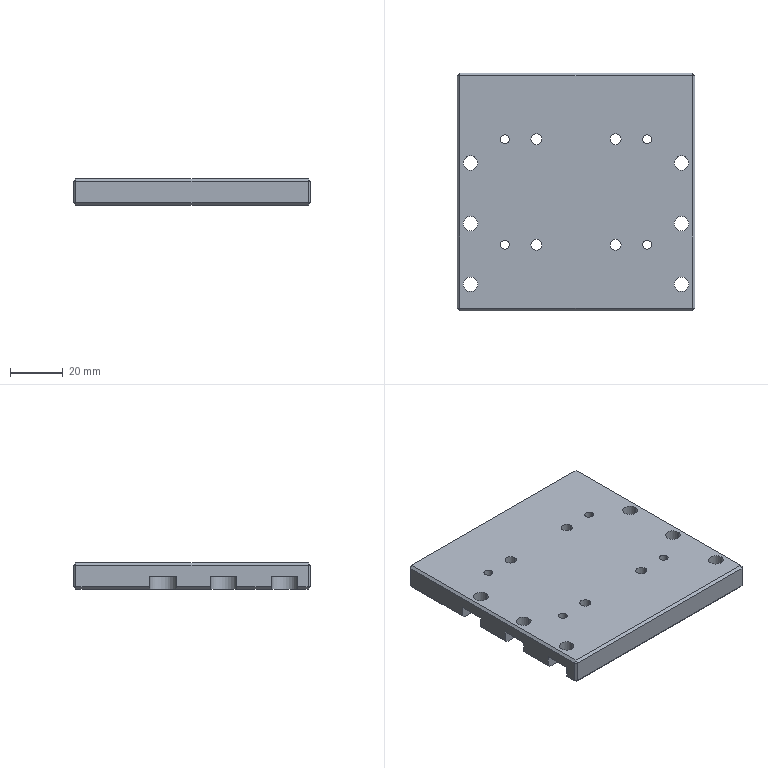Part | STEP file | 02-05 camera fixing plate | 1 solid | 87 faces | box 90 x 90 x 10 mm | volume 76368 mm3 | plane 50 | cylinder 37 | commonest cylinder face diameters 5.5 x12 10 x9 3.3 x8 4.2 x8